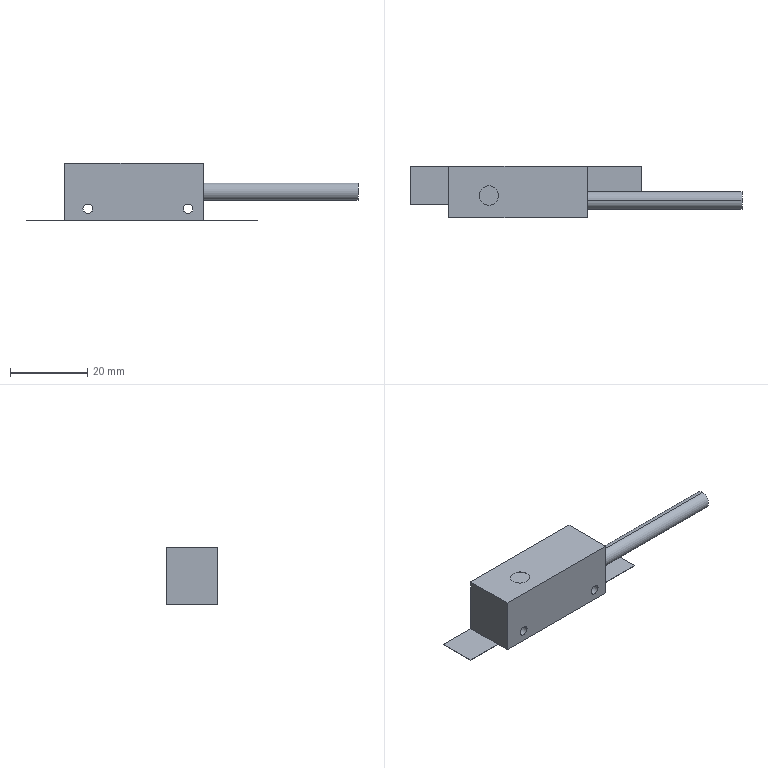Part | SolidWorks | features BaseBody 2 | 2 solids | 27 faces | box 86 x 13.4 x 14.9 mm | volume 7701 mm3 | plane 19 | cylinder 8 | commonest cylinder face diameters 2.5 x4 4.5 x2 5 x2
STEP:
#1=CARTESIAN_POINT('',(32.,6.7,0.));
#2=VERTEX_POINT('',#1);
#3=CARTESIAN_POINT('',(32.,-3.3,0.));
#4=VERTEX_POINT('',#3);
#5=CARTESIAN_POINT('',(32.,1.7,0.));
#6=DIRECTION('',(0.,-1.,0.));
#7=VECTOR('',#6,1000.);
#8=LINE('',#5,#7);
#9=EDGE_CURVE('',#2,#4,#8,.T.);
#10=ORIENTED_EDGE('',*,*,#9,.F.);
#11=CARTESIAN_POINT('',(-28.,6.7,0.));
#12=VERTEX_POINT('',#11);
#13=CARTESIAN_POINT('',(2.,6.7,0.));
#14=DIRECTION('',(1.,0.,0.));
#15=VECTOR('',#14,1000.);
#16=LINE('',#13,#15);
#17=EDGE_CURVE('',#12,#2,#16,.T.);
#18=ORIENTED_EDGE('',*,*,#17,.F.);
#19=CARTESIAN_POINT('',(-28.,-3.3,0.));
#20=VERTEX_POINT('',#19);
#21=CARTESIAN_POINT('',(-28.,1.7,0.));
#22=DIRECTION('',(0.,1.,0.));
#23=VECTOR('',#22,1000.);
#24=LINE('',#21,#23);
#25=EDGE_CURVE('',#20,#12,#24,.T.);
#26=ORIENTED_EDGE('',*,*,#25,.F.);
#27=CARTESIAN_POINT('',(2.,-3.3,0.));
#28=DIRECTION('',(-1.,0.,0.));
#29=VECTOR('',#28,1000.);
#30=LINE('',#27,#29);
#31=EDGE_CURVE('',#4,#20,#30,.T.);
#32=ORIENTED_EDGE('',*,*,#31,.F.);
#33=EDGE_LOOP('',(#10,#18,#26,#32));
#34=FACE_OUTER_BOUND('',#33,.T.);
#35=CARTESIAN_POINT('',(32.,-3.3,0.));
#36=DIRECTION('',(0.,0.,-1.));
#37=DIRECTION('',(-1.,0.,0.));
#38=AXIS2_PLACEMENT_3D('',#35,#36,#37);
#39=PLANE('',#38);
#40=ADVANCED_FACE('',(#34),#39,.F.);
#41=CARTESIAN_POINT('',(32.,-3.3,-0.1));
#42=VERTEX_POINT('',#41);
#43=CARTESIAN_POINT('',(-28.,-3.3,-0.1));
#44=VERTEX_POINT('',#43);
#45=CARTESIAN_POINT('',(2.,-3.3,-0.1));
#46=DIRECTION('',(-1.,0.,0.));
#47=VECTOR('',#46,1000.);
#48=LINE('',#45,#47);
#49=EDGE_CURVE('',#42,#44,#48,.T.);
#50=ORIENTED_EDGE('',*,*,#49,.F.);
#51=CARTESIAN_POINT('',(32.,-3.3,-0.05));
#52=DIRECTION('',(0.,0.,-1.));
#53=VECTOR('',#52,1000.);
#54=LINE('',#51,#53);
#55=EDGE_CURVE('',#4,#42,#54,.T.);
#56=ORIENTED_EDGE('',*,*,#55,.F.);
#57=ORIENTED_EDGE('',*,*,#31,.T.);
#58=CARTESIAN_POINT('',(-28.,-3.3,-0.05));
#59=DIRECTION('',(0.,0.,1.));
#60=VECTOR('',#59,1000.);
#61=LINE('',#58,#60);
#62=EDGE_CURVE('',#44,#20,#61,.T.);
#63=ORIENTED_EDGE('',*,*,#62,.F.);
#64=EDGE_LOOP('',(#50,#56,#57,#63));
#65=FACE_OUTER_BOUND('',#64,.T.);
#66=CARTESIAN_POINT('',(32.,-3.3,-0.1));
#67=DIRECTION('',(0.,1.,0.));
#68=DIRECTION('',(-1.,0.,0.));
#69=AXIS2_PLACEMENT_3D('',#66,#67,#68);
#70=PLANE('',#69);
#71=ADVANCED_FACE('',(#65),#70,.F.);
#72=CARTESIAN_POINT('',(32.,6.7,-0.1));
#73=VERTEX_POINT('',#72);
#74=CARTESIAN_POINT('',(32.,1.7,-0.1));
#75=DIRECTION('',(0.,-1.,0.));
#76=VECTOR('',#75,1000.);
#77=LINE('',#74,#76);
#78=EDGE_CURVE('',#73,#42,#77,.T.);
#79=ORIENTED_EDGE('',*,*,#78,.F.);
#80=CARTESIAN_POINT('',(32.,6.7,-0.05));
#81=DIRECTION('',(0.,0.,-1.));
#82=VECTOR('',#81,1000.);
#83=LINE('',#80,#82);
#84=EDGE_CURVE('',#2,#73,#83,.T.);
#85=ORIENTED_EDGE('',*,*,#84,.F.);
#86=ORIENTED_EDGE('',*,*,#9,.T.);
#87=ORIENTED_EDGE('',*,*,#55,.T.);
#88=EDGE_LOOP('',(#79,#85,#86,#87));
#89=FACE_OUTER_BOUND('',#88,.T.);
#90=CARTESIAN_POINT('',(32.,-3.3,-0.1));
#91=DIRECTION('',(-1.,0.,0.));
#92=DIRECTION('',(0.,0.,1.));
#93=AXIS2_PLACEMENT_3D('',#90,#91,#92);
#94=PLANE('',#93);
#95=ADVANCED_FACE('',(#89),#94,.F.);
#96=CARTESIAN_POINT('',(-28.,6.7,-0.1));
#97=VERTEX_POINT('',#96);
#98=CARTESIAN_POINT('',(2.,6.7,-0.1));
#99=DIRECTION('',(1.,0.,0.));
#100=VECTOR('',#99,1000.);
#101=LINE('',#98,#100);
#102=EDGE_CURVE('',#97,#73,#101,.T.);
#103=ORIENTED_EDGE('',*,*,#102,.F.);
#104=CARTESIAN_POINT('',(-28.,6.7,-0.05));
#105=DIRECTION('',(0.,0.,-1.));
#106=VECTOR('',#105,1000.);
#107=LINE('',#104,#106);
#108=EDGE_CURVE('',#12,#97,#107,.T.);
#109=ORIENTED_EDGE('',*,*,#108,.F.);
#110=ORIENTED_EDGE('',*,*,#17,.T.);
#111=ORIENTED_EDGE('',*,*,#84,.T.);
#112=EDGE_LOOP('',(#103,#109,#110,#111));
#113=FACE_OUTER_BOUND('',#112,.T.);
#114=CARTESIAN_POINT('',(-28.,6.7,-0.1));
#115=DIRECTION('',(0.,-1.,0.));
#116=DIRECTION('',(1.,0.,0.));
#117=AXIS2_PLACEMENT_3D('',#114,#115,#116);
#118=PLANE('',#117);
#119=ADVANCED_FACE('',(#113),#118,.F.);
#120=CARTESIAN_POINT('',(-28.,1.7,-0.1));
#121=DIRECTION('',(0.,1.,0.));
#122=VECTOR('',#121,1000.);
#123=LINE('',#120,#122);
#124=EDGE_CURVE('',#44,#97,#123,.T.);
#125=ORIENTED_EDGE('',*,*,#124,.F.);
#126=ORIENTED_EDGE('',*,*,#62,.T.);
#127=ORIENTED_EDGE('',*,*,#25,.T.);
#128=ORIENTED_EDGE('',*,*,#108,.T.);
#129=EDGE_LOOP('',(#125,#126,#127,#128));
#130=FACE_OUTER_BOUND('',#129,.T.);
#131=CARTESIAN_POINT('',(-28.,-3.3,0.));
#132=DIRECTION('',(1.,0.,0.));
#133=DIRECTION('',(0.,0.,-1.));
#134=AXIS2_PLACEMENT_3D('',#131,#132,#133);
#135=PLANE('',#134);
#136=ADVANCED_FACE('',(#130),#135,.F.);
#137=ORIENTED_EDGE('',*,*,#124,.T.);
#138=ORIENTED_EDGE('',*,*,#102,.T.);
#139=ORIENTED_EDGE('',*,*,#78,.T.);
#140=ORIENTED_EDGE('',*,*,#49,.T.);
#141=EDGE_LOOP('',(#137,#138,#139,#140));
#142=FACE_OUTER_BOUND('',#141,.T.);
#143=CARTESIAN_POINT('',(32.,-3.3,-0.1));
#144=DIRECTION('',(0.,0.,-1.));
#145=DIRECTION('',(-1.,0.,0.));
#146=AXIS2_PLACEMENT_3D('',#143,#144,#145);
#147=PLANE('',#146);
#148=ADVANCED_FACE('',(#142),#147,.T.);
#149=CLOSED_SHELL('',(#40,#71,#95,#119,#136,#148));
#150=MANIFOLD_SOLID_BREP('',#149);
#151=CARTESIAN_POINT('',(-5.051,-0.9311,14.7));
#152=VERTEX_POINT('',#151);
#153=CARTESIAN_POINT('',(-10.051,-0.9311,14.7));
#154=VERTEX_POINT('',#153);
#155=CARTESIAN_POINT('',(-7.551,-0.9311,14.7));
#156=DIRECTION('',(0.,0.,-1.));
#157=DIRECTION('',(1.,0.,0.));
#158=AXIS2_PLACEMENT_3D('',#155,#156,#157);
#159=CIRCLE('',#158,2.5);
#160=EDGE_CURVE('',#152,#154,#159,.T.);
#161=ORIENTED_EDGE('',*,*,#160,.T.);
#162=CARTESIAN_POINT('',(-10.051,-0.9311,14.8));
#163=VERTEX_POINT('',#162);
#164=CARTESIAN_POINT('',(-10.051,-0.9311,14.7));
#165=DIRECTION('',(0.,0.,1.));
#166=VECTOR('',#165,1000.);
#167=LINE('',#164,#166);
#168=EDGE_CURVE('',#154,#163,#167,.T.);
#169=ORIENTED_EDGE('',*,*,#168,.T.);
#170=CARTESIAN_POINT('',(-5.051,-0.9311,14.8));
#171=VERTEX_POINT('',#170);
#172=CARTESIAN_POINT('',(-7.551,-0.9311,14.8));
#173=DIRECTION('',(0.,0.,1.));
#174=DIRECTION('',(1.,0.,0.));
#175=AXIS2_PLACEMENT_3D('',#172,#173,#174);
#176=CIRCLE('',#175,2.5);
#177=EDGE_CURVE('',#163,#171,#176,.T.);
#178=ORIENTED_EDGE('',*,*,#177,.T.);
#179=CARTESIAN_POINT('',(-5.051,-0.9311,14.7));
#180=DIRECTION('',(0.,0.,1.));
#181=VECTOR('',#180,1000.);
#182=LINE('',#179,#181);
#183=EDGE_CURVE('',#152,#171,#182,.T.);
#184=ORIENTED_EDGE('',*,*,#183,.F.);
#185=EDGE_LOOP('',(#161,#169,#178,#184));
#186=FACE_OUTER_BOUND('',#185,.T.);
#187=CARTESIAN_POINT('',(-7.551,-0.9311,14.7));
#188=DIRECTION('',(0.,0.,1.));
#189=DIRECTION('',(1.,0.,0.));
#190=AXIS2_PLACEMENT_3D('',#187,#188,#189);
#191=CYLINDRICAL_SURFACE('',#190,2.5);
#192=ADVANCED_FACE('',(#186),#191,.F.);
#193=CARTESIAN_POINT('',(12.75,-6.7,3.));
#194=VERTEX_POINT('',#193);
#195=CARTESIAN_POINT('',(15.25,-6.7,3.));
#196=VERTEX_POINT('',#195);
#197=CARTESIAN_POINT('',(14.,-6.7,3.));
#198=DIRECTION('',(0.,-1.,0.));
#199=DIRECTION('',(-1.,0.,0.));
#200=AXIS2_PLACEMENT_3D('',#197,#198,#199);
#201=CIRCLE('',#200,1.25);
#202=EDGE_CURVE('',#194,#196,#201,.T.);
#203=ORIENTED_EDGE('',*,*,#202,.T.);
#204=CARTESIAN_POINT('',(15.25,6.7,3.));
#205=VERTEX_POINT('',#204);
#206=CARTESIAN_POINT('',(15.25,-6.7,3.));
#207=DIRECTION('',(0.,1.,0.));
#208=VECTOR('',#207,1000.);
#209=LINE('',#206,#208);
#210=EDGE_CURVE('',#196,#205,#209,.T.);
#211=ORIENTED_EDGE('',*,*,#210,.T.);
#212=CARTESIAN_POINT('',(12.75,6.7,3.));
#213=VERTEX_POINT('',#212);
#214=CARTESIAN_POINT('',(14.,6.7,3.));
#215=DIRECTION('',(0.,1.,0.));
#216=DIRECTION('',(-1.,0.,0.));
#217=AXIS2_PLACEMENT_3D('',#214,#215,#216);
#218=CIRCLE('',#217,1.25);
#219=EDGE_CURVE('',#205,#213,#218,.T.);
#220=ORIENTED_EDGE('',*,*,#219,.T.);
#221=CARTESIAN_POINT('',(12.75,-6.7,3.));
#222=DIRECTION('',(0.,1.,0.));
#223=VECTOR('',#222,1000.);
#224=LINE('',#221,#223);
#225=EDGE_CURVE('',#194,#213,#224,.T.);
#226=ORIENTED_EDGE('',*,*,#225,.F.);
#227=EDGE_LOOP('',(#203,#211,#220,#226));
#228=FACE_OUTER_BOUND('',#227,.T.);
#229=CARTESIAN_POINT('',(14.,-6.7,3.));
#230=DIRECTION('',(0.,1.,0.));
#231=DIRECTION('',(-1.,0.,0.));
#232=AXIS2_PLACEMENT_3D('',#229,#230,#231);
#233=CYLINDRICAL_SURFACE('',#232,1.25);
#234=ADVANCED_FACE('',(#228),#233,.F.);
#235=CARTESIAN_POINT('',(-13.25,-6.7,3.));
#236=VERTEX_POINT('',#235);
#237=CARTESIAN_POINT('',(-10.75,-6.7,3.));
#238=VERTEX_POINT('',#237);
#239=CARTESIAN_POINT('',(-12.,-6.7,3.));
#240=DIRECTION('',(0.,-1.,0.));
#241=DIRECTION('',(-1.,0.,0.));
#242=AXIS2_PLACEMENT_3D('',#239,#240,#241);
#243=CIRCLE('',#242,1.25);
#244=EDGE_CURVE('',#236,#238,#243,.T.);
#245=ORIENTED_EDGE('',*,*,#244,.T.);
#246=CARTESIAN_POINT('',(-10.75,6.7,3.));
#247=VERTEX_POINT('',#246);
#248=CARTESIAN_POINT('',(-10.75,-6.7,3.));
#249=DIRECTION('',(0.,1.,0.));
#250=VECTOR('',#249,1000.);
#251=LINE('',#248,#250);
#252=EDGE_CURVE('',#238,#247,#251,.T.);
#253=ORIENTED_EDGE('',*,*,#252,.T.);
#254=CARTESIAN_POINT('',(-13.25,6.7,3.));
#255=VERTEX_POINT('',#254);
#256=CARTESIAN_POINT('',(-12.,6.7,3.));
#257=DIRECTION('',(0.,1.,0.));
#258=DIRECTION('',(-1.,0.,0.));
#259=AXIS2_PLACEMENT_3D('',#256,#257,#258);
#260=CIRCLE('',#259,1.25);
#261=EDGE_CURVE('',#247,#255,#260,.T.);
#262=ORIENTED_EDGE('',*,*,#261,.T.);
#263=CARTESIAN_POINT('',(-13.25,-6.7,3.));
#264=DIRECTION('',(0.,1.,0.));
#265=VECTOR('',#264,1000.);
#266=LINE('',#263,#265);
#267=EDGE_CURVE('',#236,#255,#266,.T.);
#268=ORIENTED_EDGE('',*,*,#267,.F.);
#269=EDGE_LOOP('',(#245,#253,#262,#268));
#270=FACE_OUTER_BOUND('',#269,.T.);
#271=CARTESIAN_POINT('',(-12.,-6.7,3.));
#272=DIRECTION('',(0.,1.,0.));
#273=DIRECTION('',(-1.,0.,0.));
#274=AXIS2_PLACEMENT_3D('',#271,#272,#273);
#275=CYLINDRICAL_SURFACE('',#274,1.25);
#276=ADVANCED_FACE('',(#270),#275,.F.);
#277=CARTESIAN_POINT('',(58.,-2.2,5.15));
#278=VERTEX_POINT('',#277);
#279=CARTESIAN_POINT('',(58.,-2.2,9.65));
#280=VERTEX_POINT('',#279);
#281=CARTESIAN_POINT('',(58.,-2.2,7.4));
#282=DIRECTION('',(1.,0.,0.));
#283=DIRECTION('',(0.,0.,1.));
#284=AXIS2_PLACEMENT_3D('',#281,#282,#283);
#285=CIRCLE('',#284,2.25);
#286=EDGE_CURVE('',#278,#280,#285,.T.);
#287=ORIENTED_EDGE('',*,*,#286,.F.);
#288=CARTESIAN_POINT('',(18.,-2.2,5.15));
#289=VERTEX_POINT('',#288);
#290=CARTESIAN_POINT('',(58.,-2.2,5.15));
#291=DIRECTION('',(-1.,0.,0.));
#292=VECTOR('',#291,1000.);
#293=LINE('',#290,#292);
#294=EDGE_CURVE('',#278,#289,#293,.T.);
#295=ORIENTED_EDGE('',*,*,#294,.T.);
#296=CARTESIAN_POINT('',(18.,-2.2,9.65));
#297=VERTEX_POINT('',#296);
#298=CARTESIAN_POINT('',(18.,-2.2,7.4));
#299=DIRECTION('',(1.,0.,0.));
#300=DIRECTION('',(0.,0.,1.));
#301=AXIS2_PLACEMENT_3D('',#298,#299,#300);
#302=CIRCLE('',#301,2.25);
#303=EDGE_CURVE('',#289,#297,#302,.T.);
#304=ORIENTED_EDGE('',*,*,#303,.T.);
#305=CARTESIAN_POINT('',(58.,-2.2,9.65));
#306=DIRECTION('',(-1.,0.,0.));
#307=VECTOR('',#306,1000.);
#308=LINE('',#305,#307);
#309=EDGE_CURVE('',#280,#297,#308,.T.);
#310=ORIENTED_EDGE('',*,*,#309,.F.);
#311=EDGE_LOOP('',(#287,#295,#304,#310));
#312=FACE_OUTER_BOUND('',#311,.T.);
#313=CARTESIAN_POINT('',(58.,-2.2,7.4));
#314=DIRECTION('',(-1.,0.,0.));
#315=DIRECTION('',(0.,0.,1.));
#316=AXIS2_PLACEMENT_3D('',#313,#314,#315);
#317=CYLINDRICAL_SURFACE('',#316,2.25);
#318=ADVANCED_FACE('',(#312),#317,.T.);
#319=ORIENTED_EDGE('',*,*,#168,.F.);
#320=CARTESIAN_POINT('',(-7.551,-0.9311,14.7));
#321=DIRECTION('',(0.,0.,-1.));
#322=DIRECTION('',(1.,0.,0.));
#323=AXIS2_PLACEMENT_3D('',#320,#321,#322);
#324=CIRCLE('',#323,2.5);
#325=EDGE_CURVE('',#154,#152,#324,.T.);
#326=ORIENTED_EDGE('',*,*,#325,.T.);
#327=ORIENTED_EDGE('',*,*,#183,.T.);
#328=CARTESIAN_POINT('',(-7.551,-0.9311,14.8));
#329=DIRECTION('',(0.,0.,1.));
#330=DIRECTION('',(1.,0.,0.));
#331=AXIS2_PLACEMENT_3D('',#328,#329,#330);
#332=CIRCLE('',#331,2.5);
#333=EDGE_CURVE('',#171,#163,#332,.T.);
#334=ORIENTED_EDGE('',*,*,#333,.T.);
#335=EDGE_LOOP('',(#319,#326,#327,#334));
#336=FACE_OUTER_BOUND('',#335,.T.);
#337=CARTESIAN_POINT('',(-7.551,-0.9311,14.7));
#338=DIRECTION('',(0.,0.,1.));
#339=DIRECTION('',(1.,0.,0.));
#340=AXIS2_PLACEMENT_3D('',#337,#338,#339);
#341=CYLINDRICAL_SURFACE('',#340,2.5);
#342=ADVANCED_FACE('',(#336),#341,.F.);
#343=ORIENTED_EDGE('',*,*,#333,.F.);
#344=ORIENTED_EDGE('',*,*,#177,.F.);
#345=EDGE_LOOP('',(#343,#344));
#346=FACE_BOUND('',#345,.T.);
#347=CARTESIAN_POINT('',(18.,-6.7,14.8));
#348=VERTEX_POINT('',#347);
#349=CARTESIAN_POINT('',(18.,6.7,14.8));
#350=VERTEX_POINT('',#349);
#351=CARTESIAN_POINT('',(18.,0.,14.8));
#352=DIRECTION('',(0.,1.,0.));
#353=VECTOR('',#352,1000.);
#354=LINE('',#351,#353);
#355=EDGE_CURVE('',#348,#350,#354,.T.);
#356=ORIENTED_EDGE('',*,*,#355,.T.);
#357=CARTESIAN_POINT('',(-18.,6.7,14.8));
#358=VERTEX_POINT('',#357);
#359=CARTESIAN_POINT('',(0.,6.7,14.8));
#360=DIRECTION('',(-1.,0.,0.));
#361=VECTOR('',#360,1000.);
#362=LINE('',#359,#361);
#363=EDGE_CURVE('',#350,#358,#362,.T.);
#364=ORIENTED_EDGE('',*,*,#363,.T.);
#365=CARTESIAN_POINT('',(-18.,-6.7,14.8));
#366=VERTEX_POINT('',#365);
#367=CARTESIAN_POINT('',(-18.,0.,14.8));
#368=DIRECTION('',(0.,-1.,0.));
#369=VECTOR('',#368,1000.);
#370=LINE('',#367,#369);
#371=EDGE_CURVE('',#358,#366,#370,.T.);
#372=ORIENTED_EDGE('',*,*,#371,.T.);
#373=CARTESIAN_POINT('',(0.,-6.7,14.8));
#374=DIRECTION('',(1.,0.,0.));
#375=VECTOR('',#374,1000.);
#376=LINE('',#373,#375);
#377=EDGE_CURVE('',#366,#348,#376,.T.);
#378=ORIENTED_EDGE('',*,*,#377,.T.);
#379=EDGE_LOOP('',(#356,#364,#372,#378));
#380=FACE_OUTER_BOUND('',#379,.T.);
#381=CARTESIAN_POINT('',(-18.,-6.7,14.8));
#382=DIRECTION('',(0.,0.,1.));
#383=DIRECTION('',(1.,0.,0.));
#384=AXIS2_PLACEMENT_3D('',#381,#382,#383);
#385=PLANE('',#384);
#386=ADVANCED_FACE('',(#346,#380),#385,.T.);
#387=ORIENTED_EDGE('',*,*,#160,.F.);
#388=ORIENTED_EDGE('',*,*,#325,.F.);
#389=EDGE_LOOP('',(#387,#388));
#390=FACE_OUTER_BOUND('',#389,.T.);
#391=CARTESIAN_POINT('',(-10.081,-3.461,14.7));
#392=DIRECTION('',(0.,0.,1.));
#393=DIRECTION('',(1.,0.,0.));
#394=AXIS2_PLACEMENT_3D('',#391,#392,#393);
#395=PLANE('',#394);
#396=ADVANCED_FACE('',(#390),#395,.T.);
#397=CARTESIAN_POINT('',(14.,6.7,3.));
#398=DIRECTION('',(0.,1.,0.));
#399=DIRECTION('',(-1.,0.,0.));
#400=AXIS2_PLACEMENT_3D('',#397,#398,#399);
#401=CIRCLE('',#400,1.25);
#402=EDGE_CURVE('',#213,#205,#401,.T.);
#403=ORIENTED_EDGE('',*,*,#402,.F.);
#404=ORIENTED_EDGE('',*,*,#219,.F.);
#405=EDGE_LOOP('',(#403,#404));
#406=FACE_BOUND('',#405,.T.);
#407=CARTESIAN_POINT('',(-12.,6.7,3.));
#408=DIRECTION('',(0.,1.,0.));
#409=DIRECTION('',(-1.,0.,0.));
#410=AXIS2_PLACEMENT_3D('',#407,#408,#409);
#411=CIRCLE('',#410,1.25);
#412=EDGE_CURVE('',#255,#247,#411,.T.);
#413=ORIENTED_EDGE('',*,*,#412,.F.);
#414=ORIENTED_EDGE('',*,*,#261,.F.);
#415=EDGE_LOOP('',(#413,#414));
#416=FACE_BOUND('',#415,.T.);
#417=ORIENTED_EDGE('',*,*,#363,.F.);
#418=CARTESIAN_POINT('',(18.,6.7,0.));
#419=VERTEX_POINT('',#418);
#420=CARTESIAN_POINT('',(18.,6.7,7.4));
#421=DIRECTION('',(0.,0.,1.));
#422=VECTOR('',#421,1000.);
#423=LINE('',#420,#422);
#424=EDGE_CURVE('',#419,#350,#423,.T.);
#425=ORIENTED_EDGE('',*,*,#424,.F.);
#426=CARTESIAN_POINT('',(-18.,6.7,0.));
#427=VERTEX_POINT('',#426);
#428=CARTESIAN_POINT('',(0.,6.7,0.));
#429=DIRECTION('',(1.,0.,0.));
#430=VECTOR('',#429,1000.);
#431=LINE('',#428,#430);
#432=EDGE_CURVE('',#427,#419,#431,.T.);
#433=ORIENTED_EDGE('',*,*,#432,.F.);
#434=CARTESIAN_POINT('',(-18.,6.7,7.4));
#435=DIRECTION('',(0.,0.,-1.));
#436=VECTOR('',#435,1000.);
#437=LINE('',#434,#436);
#438=EDGE_CURVE('',#358,#427,#437,.T.);
#439=ORIENTED_EDGE('',*,*,#438,.F.);
#440=EDGE_LOOP('',(#417,#425,#433,#439));
#441=FACE_OUTER_BOUND('',#440,.T.);
#442=CARTESIAN_POINT('',(-18.,6.7,14.8));
#443=DIRECTION('',(0.,-1.,0.));
#444=DIRECTION('',(0.,0.,-1.));
#445=AXIS2_PLACEMENT_3D('',#442,#443,#444);
#446=PLANE('',#445);
#447=ADVANCED_FACE('',(#406,#416,#441),#446,.F.);
#448=CARTESIAN_POINT('',(18.,-2.2,7.4));
#449=DIRECTION('',(1.,0.,0.));
#450=DIRECTION('',(0.,0.,1.));
#451=AXIS2_PLACEMENT_3D('',#448,#449,#450);
#452=CIRCLE('',#451,2.25);
#453=EDGE_CURVE('',#297,#289,#452,.T.);
#454=ORIENTED_EDGE('',*,*,#453,.F.);
#455=ORIENTED_EDGE('',*,*,#303,.F.);
#456=EDGE_LOOP('',(#454,#455));
#457=FACE_BOUND('',#456,.T.);
#458=ORIENTED_EDGE('',*,*,#355,.F.);
#459=CARTESIAN_POINT('',(18.,-6.7,0.));
#460=VERTEX_POINT('',#459);
#461=CARTESIAN_POINT('',(18.,-6.7,7.4));
#462=DIRECTION('',(0.,0.,1.));
#463=VECTOR('',#462,1000.);
#464=LINE('',#461,#463);
#465=EDGE_CURVE('',#460,#348,#464,.T.);
#466=ORIENTED_EDGE('',*,*,#465,.F.);
#467=CARTESIAN_POINT('',(18.,0.,0.));
#468=DIRECTION('',(0.,-1.,0.));
#469=VECTOR('',#468,1000.);
#470=LINE('',#467,#469);
#471=EDGE_CURVE('',#419,#460,#470,.T.);
#472=ORIENTED_EDGE('',*,*,#471,.F.);
#473=ORIENTED_EDGE('',*,*,#424,.T.);
#474=EDGE_LOOP('',(#458,#466,#472,#473));
#475=FACE_OUTER_BOUND('',#474,.T.);
#476=CARTESIAN_POINT('',(18.,-6.7,0.));
#477=DIRECTION('',(-1.,0.,0.));
#478=DIRECTION('',(0.,0.,1.));
#479=AXIS2_PLACEMENT_3D('',#476,#477,#478);
#480=PLANE('',#479);
#481=ADVANCED_FACE('',(#457,#475),#480,.F.);
#482=ORIENTED_EDGE('',*,*,#202,.F.);
#483=CARTESIAN_POINT('',(14.,-6.7,3.));
#484=DIRECTION('',(0.,-1.,0.));
#485=DIRECTION('',(-1.,0.,0.));
#486=AXIS2_PLACEMENT_3D('',#483,#484,#485);
#487=CIRCLE('',#486,1.25);
#488=EDGE_CURVE('',#196,#194,#487,.T.);
#489=ORIENTED_EDGE('',*,*,#488,.F.);
#490=EDGE_LOOP('',(#482,#489));
#491=FACE_BOUND('',#490,.T.);
#492=ORIENTED_EDGE('',*,*,#244,.F.);
#493=CARTESIAN_POINT('',(-12.,-6.7,3.));
#494=DIRECTION('',(0.,-1.,0.));
#495=DIRECTION('',(-1.,0.,0.));
#496=AXIS2_PLACEMENT_3D('',#493,#494,#495);
#497=CIRCLE('',#496,1.25);
#498=EDGE_CURVE('',#238,#236,#497,.T.);
#499=ORIENTED_EDGE('',*,*,#498,.F.);
#500=EDGE_LOOP('',(#492,#499));
#501=FACE_BOUND('',#500,.T.);
#502=ORIENTED_EDGE('',*,*,#377,.F.);
#503=CARTESIAN_POINT('',(-18.,-6.7,0.));
#504=VERTEX_POINT('',#503);
#505=CARTESIAN_POINT('',(-18.,-6.7,7.4));
#506=DIRECTION('',(0.,0.,1.));
#507=VECTOR('',#506,1000.);
#508=LINE('',#505,#507);
#509=EDGE_CURVE('',#504,#366,#508,.T.);
#510=ORIENTED_EDGE('',*,*,#509,.F.);
#511=CARTESIAN_POINT('',(0.,-6.7,0.));
#512=DIRECTION('',(-1.,0.,0.));
#513=VECTOR('',#512,1000.);
#514=LINE('',#511,#513);
#515=EDGE_CURVE('',#460,#504,#514,.T.);
#516=ORIENTED_EDGE('',*,*,#515,.F.);
#517=ORIENTED_EDGE('',*,*,#465,.T.);
#518=EDGE_LOOP('',(#502,#510,#516,#517));
#519=FACE_OUTER_BOUND('',#518,.T.);
#520=CARTESIAN_POINT('',(-18.,-6.7,0.));
#521=DIRECTION('',(0.,1.,0.));
#522=DIRECTION('',(0.,0.,1.));
#523=AXIS2_PLACEMENT_3D('',#520,#521,#522);
#524=PLANE('',#523);
#525=ADVANCED_FACE('',(#491,#501,#519),#524,.F.);
#526=ORIENTED_EDGE('',*,*,#371,.F.);
#527=ORIENTED_EDGE('',*,*,#438,.T.);
#528=CARTESIAN_POINT('',(-18.,0.,0.));
#529=DIRECTION('',(0.,1.,0.));
#530=VECTOR('',#529,1000.);
#531=LINE('',#528,#530);
#532=EDGE_CURVE('',#504,#427,#531,.T.);
#533=ORIENTED_EDGE('',*,*,#532,.F.);
#534=ORIENTED_EDGE('',*,*,#509,.T.);
#535=EDGE_LOOP('',(#526,#527,#533,#534));
#536=FACE_OUTER_BOUND('',#535,.T.);
#537=CARTESIAN_POINT('',(-18.,-6.7,14.8));
#538=DIRECTION('',(1.,0.,0.));
#539=DIRECTION('',(0.,0.,-1.));
#540=AXIS2_PLACEMENT_3D('',#537,#538,#539);
#541=PLANE('',#540);
#542=ADVANCED_FACE('',(#536),#541,.F.);
#543=ORIENTED_EDGE('',*,*,#210,.F.);
#544=ORIENTED_EDGE('',*,*,#488,.T.);
#545=ORIENTED_EDGE('',*,*,#225,.T.);
#546=ORIENTED_EDGE('',*,*,#402,.T.);
#547=EDGE_LOOP('',(#543,#544,#545,#546));
#548=FACE_OUTER_BOUND('',#547,.T.);
#549=CARTESIAN_POINT('',(14.,-6.7,3.));
#550=DIRECTION('',(0.,1.,0.));
#551=DIRECTION('',(-1.,0.,0.));
#552=AXIS2_PLACEMENT_3D('',#549,#550,#551);
#553=CYLINDRICAL_SURFACE('',#552,1.25);
#554=ADVANCED_FACE('',(#548),#553,.F.);
#555=ORIENTED_EDGE('',*,*,#252,.F.);
#556=ORIENTED_EDGE('',*,*,#498,.T.);
#557=ORIENTED_EDGE('',*,*,#267,.T.);
#558=ORIENTED_EDGE('',*,*,#412,.T.);
#559=EDGE_LOOP('',(#555,#556,#557,#558));
#560=FACE_OUTER_BOUND('',#559,.T.);
#561=CARTESIAN_POINT('',(-12.,-6.7,3.));
#562=DIRECTION('',(0.,1.,0.));
#563=DIRECTION('',(-1.,0.,0.));
#564=AXIS2_PLACEMENT_3D('',#561,#562,#563);
#565=CYLINDRICAL_SURFACE('',#564,1.25);
#566=ADVANCED_FACE('',(#560),#565,.F.);
#567=CARTESIAN_POINT('',(-3.,0.1,0.));
#568=VERTEX_POINT('',#567);
#569=CARTESIAN_POINT('',(-7.,0.1,0.));
#570=VERTEX_POINT('',#569);
#571=CARTESIAN_POINT('',(0.,0.1,0.));
#572=DIRECTION('',(-1.,0.,0.));
#573=VECTOR('',#572,1000.);
#574=LINE('',#571,#573);
#575=EDGE_CURVE('',#568,#570,#574,.T.);
#576=ORIENTED_EDGE('',*,*,#575,.F.);
#577=CARTESIAN_POINT('',(-3.,4.1,0.));
#578=VERTEX_POINT('',#577);
#579=CARTESIAN_POINT('',(-3.,0.,0.));
#580=DIRECTION('',(0.,-1.,0.));
#581=VECTOR('',#580,1000.);
#582=LINE('',#579,#581);
#583=EDGE_CURVE('',#578,#568,#582,.T.);
#584=ORIENTED_EDGE('',*,*,#583,.F.);
#585=CARTESIAN_POINT('',(-7.,4.1,0.));
#586=VERTEX_POINT('',#585);
#587=CARTESIAN_POINT('',(0.,4.1,0.));
#588=DIRECTION('',(1.,0.,0.));
#589=VECTOR('',#588,1000.);
#590=LINE('',#587,#589);
#591=EDGE_CURVE('',#586,#578,#590,.T.);
#592=ORIENTED_EDGE('',*,*,#591,.F.);
#593=CARTESIAN_POINT('',(-7.,0.,0.));
#594=DIRECTION('',(0.,1.,0.));
#595=VECTOR('',#594,1000.);
#596=LINE('',#593,#595);
#597=EDGE_CURVE('',#570,#586,#596,.T.);
#598=ORIENTED_EDGE('',*,*,#597,.F.);
#599=EDGE_LOOP('',(#576,#584,#592,#598));
#600=FACE_BOUND('',#599,.T.);
#601=ORIENTED_EDGE('',*,*,#532,.T.);
#602=ORIENTED_EDGE('',*,*,#432,.T.);
#603=ORIENTED_EDGE('',*,*,#471,.T.);
#604=ORIENTED_EDGE('',*,*,#515,.T.);
#605=EDGE_LOOP('',(#601,#602,#603,#604));
#606=FACE_OUTER_BOUND('',#605,.T.);
#607=CARTESIAN_POINT('',(-18.,-6.7,0.));
#608=DIRECTION('',(0.,0.,1.));
#609=DIRECTION('',(1.,0.,0.));
#610=AXIS2_PLACEMENT_3D('',#607,#608,#609);
#611=PLANE('',#610);
#612=ADVANCED_FACE('',(#600,#606),#611,.F.);
#613=ORIENTED_EDGE('',*,*,#294,.F.);
#614=CARTESIAN_POINT('',(58.,-2.2,7.4));
#615=DIRECTION('',(1.,0.,0.));
#616=DIRECTION('',(0.,0.,1.));
#617=AXIS2_PLACEMENT_3D('',#614,#615,#616);
#618=CIRCLE('',#617,2.25);
#619=EDGE_CURVE('',#280,#278,#618,.T.);
#620=ORIENTED_EDGE('',*,*,#619,.F.);
#621=ORIENTED_EDGE('',*,*,#309,.T.);
#622=ORIENTED_EDGE('',*,*,#453,.T.);
#623=EDGE_LOOP('',(#613,#620,#621,#622));
#624=FACE_OUTER_BOUND('',#623,.T.);
#625=CARTESIAN_POINT('',(58.,-2.2,7.4));
#626=DIRECTION('',(-1.,0.,0.));
#627=DIRECTION('',(0.,0.,1.));
#628=AXIS2_PLACEMENT_3D('',#625,#626,#627);
#629=CYLINDRICAL_SURFACE('',#628,2.25);
#630=ADVANCED_FACE('',(#624),#629,.T.);
#631=CARTESIAN_POINT('',(-7.,0.1,0.1));
#632=VERTEX_POINT('',#631);
#633=CARTESIAN_POINT('',(-7.,4.1,0.1));
#634=VERTEX_POINT('',#633);
#635=CARTESIAN_POINT('',(-7.,2.1,0.1));
#636=DIRECTION('',(0.,1.,0.));
#637=VECTOR('',#636,1000.);
#638=LINE('',#635,#637);
#639=EDGE_CURVE('',#632,#634,#638,.T.);
#640=ORIENTED_EDGE('',*,*,#639,.F.);
#641=CARTESIAN_POINT('',(-7.,0.1,0.05));
#642=DIRECTION('',(0.,0.,1.));
#643=VECTOR('',#642,1000.);
#644=LINE('',#641,#643);
#645=EDGE_CURVE('',#570,#632,#644,.T.);
#646=ORIENTED_EDGE('',*,*,#645,.F.);
#647=ORIENTED_EDGE('',*,*,#597,.T.);
#648=CARTESIAN_POINT('',(-7.,4.1,0.05));
#649=DIRECTION('',(0.,0.,-1.));
#650=VECTOR('',#649,1000.);
#651=LINE('',#648,#650);
#652=EDGE_CURVE('',#634,#586,#651,.T.);
#653=ORIENTED_EDGE('',*,*,#652,.F.);
#654=EDGE_LOOP('',(#640,#646,#647,#653));
#655=FACE_OUTER_BOUND('',#654,.T.);
#656=CARTESIAN_POINT('',(-7.,0.1,0.));
#657=DIRECTION('',(-1.,0.,0.));
#658=DIRECTION('',(0.,0.,1.));
#659=AXIS2_PLACEMENT_3D('',#656,#657,#658);
#660=PLANE('',#659);
#661=ADVANCED_FACE('',(#655),#660,.F.);
#662=CARTESIAN_POINT('',(-3.,0.1,0.1));
#663=VERTEX_POINT('',#662);
#664=CARTESIAN_POINT('',(-5.,0.1,0.1));
#665=DIRECTION('',(-1.,0.,0.));
#666=VECTOR('',#665,1000.);
#667=LINE('',#664,#666);
#668=EDGE_CURVE('',#663,#632,#667,.T.);
#669=ORIENTED_EDGE('',*,*,#668,.F.);
#670=CARTESIAN_POINT('',(-3.,0.1,0.05));
#671=DIRECTION('',(0.,0.,1.));
#672=VECTOR('',#671,1000.);
#673=LINE('',#670,#672);
#674=EDGE_CURVE('',#568,#663,#673,.T.);
#675=ORIENTED_EDGE('',*,*,#674,.F.);
#676=ORIENTED_EDGE('',*,*,#575,.T.);
#677=ORIENTED_EDGE('',*,*,#645,.T.);
#678=EDGE_LOOP('',(#669,#675,#676,#677));
#679=FACE_OUTER_BOUND('',#678,.T.);
#680=CARTESIAN_POINT('',(-7.,0.1,0.));
#681=DIRECTION('',(0.,-1.,0.));
#682=DIRECTION('',(1.,0.,0.));
#683=AXIS2_PLACEMENT_3D('',#680,#681,#682);
#684=PLANE('',#683);
#685=ADVANCED_FACE('',(#679),#684,.F.);
#686=CARTESIAN_POINT('',(-3.,4.1,0.1));
#687=VERTEX_POINT('',#686);
#688=CARTESIAN_POINT('',(-3.,2.1,0.1));
#689=DIRECTION('',(0.,-1.,0.));
#690=VECTOR('',#689,1000.);
#691=LINE('',#688,#690);
#692=EDGE_CURVE('',#687,#663,#691,.T.);
#693=ORIENTED_EDGE('',*,*,#692,.F.);
#694=CARTESIAN_POINT('',(-3.,4.1,0.05));
#695=DIRECTION('',(0.,0.,1.));
#696=VECTOR('',#695,1000.);
#697=LINE('',#694,#696);
#698=EDGE_CURVE('',#578,#687,#697,.T.);
#699=ORIENTED_EDGE('',*,*,#698,.F.);
#700=ORIENTED_EDGE('',*,*,#583,.T.);
#701=ORIENTED_EDGE('',*,*,#674,.T.);
#702=EDGE_LOOP('',(#693,#699,#700,#701));
#703=FACE_OUTER_BOUND('',#702,.T.);
#704=CARTESIAN_POINT('',(-3.,0.1,0.1));
#705=DIRECTION('',(1.,0.,0.));
#706=DIRECTION('',(0.,0.,-1.));
#707=AXIS2_PLACEMENT_3D('',#704,#705,#706);
#708=PLANE('',#707);
#709=ADVANCED_FACE('',(#703),#708,.F.);
#710=CARTESIAN_POINT('',(-5.,4.1,0.1));
#711=DIRECTION('',(1.,0.,0.));
#712=VECTOR('',#711,1000.);
#713=LINE('',#710,#712);
#714=EDGE_CURVE('',#634,#687,#713,.T.);
#715=ORIENTED_EDGE('',*,*,#714,.F.);
#716=ORIENTED_EDGE('',*,*,#652,.T.);
#717=ORIENTED_EDGE('',*,*,#591,.T.);
#718=ORIENTED_EDGE('',*,*,#698,.T.);
#719=EDGE_LOOP('',(#715,#716,#717,#718));
#720=FACE_OUTER_BOUND('',#719,.T.);
#721=CARTESIAN_POINT('',(-7.,4.1,0.));
#722=DIRECTION('',(0.,1.,0.));
#723=DIRECTION('',(0.,0.,1.));
#724=AXIS2_PLACEMENT_3D('',#721,#722,#723);
#725=PLANE('',#724);
#726=ADVANCED_FACE('',(#720),#725,.F.);
#727=ORIENTED_EDGE('',*,*,#619,.T.);
#728=ORIENTED_EDGE('',*,*,#286,.T.);
#729=EDGE_LOOP('',(#727,#728));
#730=FACE_OUTER_BOUND('',#729,.T.);
#731=CARTESIAN_POINT('',(58.,-4.477,9.677));
#732=DIRECTION('',(1.,0.,0.));
#733=DIRECTION('',(0.,0.,-1.));
#734=AXIS2_PLACEMENT_3D('',#731,#732,#733);
#735=PLANE('',#734);
#736=ADVANCED_FACE('',(#730),#735,.T.);
#737=ORIENTED_EDGE('',*,*,#639,.T.);
#738=ORIENTED_EDGE('',*,*,#714,.T.);
#739=ORIENTED_EDGE('',*,*,#692,.T.);
#740=ORIENTED_EDGE('',*,*,#668,.T.);
#741=EDGE_LOOP('',(#737,#738,#739,#740));
#742=FACE_OUTER_BOUND('',#741,.T.);
#743=CARTESIAN_POINT('',(-3.,0.1,0.1));
#744=DIRECTION('',(0.,0.,-1.));
#745=DIRECTION('',(-1.,0.,0.));
#746=AXIS2_PLACEMENT_3D('',#743,#744,#745);
#747=PLANE('',#746);
#748=ADVANCED_FACE('',(#742),#747,.T.);
#749=CLOSED_SHELL('',(#192,#234,#276,#318,#342,#386,#396,#447,#481,#525,#542,#554,#566,#612,#630,#661,#685,#709,#726,#736,#748));
#750=MANIFOLD_SOLID_BREP('',#749);
#751=CARTESIAN_POINT('',(0.,0.,0.));
#752=DIRECTION('',(0.,0.,1.));
#753=DIRECTION('',(1.,0.,0.));
#754=AXIS2_PLACEMENT_3D('',#751,#752,#753);
#755=(LENGTH_UNIT()NAMED_UNIT(*)SI_UNIT(.MILLI.,.METRE.));
#756=UNCERTAINTY_MEASURE_WITH_UNIT(LENGTH_MEASURE(0.00001),#755,'','');
#757=(NAMED_UNIT(*)PLANE_ANGLE_UNIT()SI_UNIT($,.RADIAN.));
#758=(NAMED_UNIT(*)SI_UNIT($,.STERADIAN.)SOLID_ANGLE_UNIT());
#759=(GEOMETRIC_REPRESENTATION_CONTEXT(3)GLOBAL_UNCERTAINTY_ASSIGNED_CONTEXT((#756))GLOBAL_UNIT_ASSIGNED_CONTEXT((#755,#757,#758))REPRESENTATION_CONTEXT('',''));
#760=ADVANCED_BREP_SHAPE_REPRESENTATION('',(#150,#750,#754),#759);